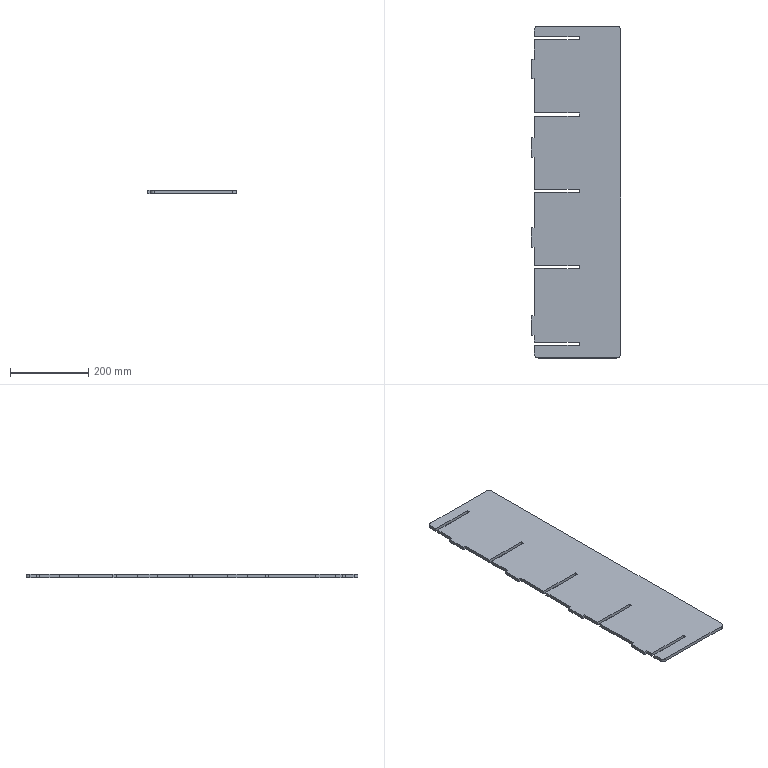Part | SolidWorks | features FlatPattern 1, SMBaseFlange 1, SheetMetal 1 | 1 solid | 46 faces | box 227.5 x 847.5 x 8 mm | volume 1466273 mm3 | plane 42 | cylinder 4 | commonest cylinder face diameters 20 x4
STEP:
#1=CARTESIAN_POINT('',(995.006,-468.438,0.));
#2=VERTEX_POINT('',#1);
#3=CARTESIAN_POINT('',(1005.006,-478.438,0.));
#4=VERTEX_POINT('',#3);
#5=CARTESIAN_POINT('',(1005.006,-468.438,0.));
#6=DIRECTION('',(0.,0.,1.));
#7=DIRECTION('',(-1.,0.,0.));
#8=AXIS2_PLACEMENT_3D('',#5,#6,#7);
#9=CIRCLE('',#8,10.);
#10=EDGE_CURVE('',#2,#4,#9,.T.);
#11=ORIENTED_EDGE('',*,*,#10,.F.);
#12=CARTESIAN_POINT('',(995.006,-468.438,-8.));
#13=VERTEX_POINT('',#12);
#14=CARTESIAN_POINT('',(995.006,-468.438,-8.));
#15=DIRECTION('',(0.,0.,1.));
#16=VECTOR('',#15,1000.);
#17=LINE('',#14,#16);
#18=EDGE_CURVE('',#13,#2,#17,.T.);
#19=ORIENTED_EDGE('',*,*,#18,.F.);
#20=CARTESIAN_POINT('',(1005.006,-478.438,-8.));
#21=VERTEX_POINT('',#20);
#22=CARTESIAN_POINT('',(1005.006,-468.438,-8.));
#23=DIRECTION('',(0.,0.,1.));
#24=DIRECTION('',(-1.,0.,0.));
#25=AXIS2_PLACEMENT_3D('',#22,#23,#24);
#26=CIRCLE('',#25,10.);
#27=EDGE_CURVE('',#13,#21,#26,.T.);
#28=ORIENTED_EDGE('',*,*,#27,.T.);
#29=CARTESIAN_POINT('',(1005.006,-478.438,-8.));
#30=DIRECTION('',(0.,0.,1.));
#31=VECTOR('',#30,1000.);
#32=LINE('',#29,#31);
#33=EDGE_CURVE('',#21,#4,#32,.T.);
#34=ORIENTED_EDGE('',*,*,#33,.T.);
#35=EDGE_LOOP('',(#11,#19,#28,#34));
#36=FACE_OUTER_BOUND('',#35,.T.);
#37=CARTESIAN_POINT('',(1005.006,-468.438,-8.));
#38=DIRECTION('',(0.,0.,1.));
#39=DIRECTION('',(1.,0.,0.));
#40=AXIS2_PLACEMENT_3D('',#37,#38,#39);
#41=CYLINDRICAL_SURFACE('',#40,10.);
#42=ADVANCED_FACE('',(#36),#41,.T.);
#43=CARTESIAN_POINT('',(995.006,-445.938,0.));
#44=VERTEX_POINT('',#43);
#45=CARTESIAN_POINT('',(995.006,-468.438,0.));
#46=DIRECTION('',(0.,-1.,0.));
#47=VECTOR('',#46,1000.);
#48=LINE('',#45,#47);
#49=EDGE_CURVE('',#44,#2,#48,.T.);
#50=ORIENTED_EDGE('',*,*,#49,.F.);
#51=CARTESIAN_POINT('',(995.006,-445.938,-8.));
#52=VERTEX_POINT('',#51);
#53=CARTESIAN_POINT('',(995.006,-445.938,-8.));
#54=DIRECTION('',(0.,0.,1.));
#55=VECTOR('',#54,1000.);
#56=LINE('',#53,#55);
#57=EDGE_CURVE('',#52,#44,#56,.T.);
#58=ORIENTED_EDGE('',*,*,#57,.F.);
#59=CARTESIAN_POINT('',(995.006,-468.438,-8.));
#60=DIRECTION('',(0.,-1.,0.));
#61=VECTOR('',#60,1000.);
#62=LINE('',#59,#61);
#63=EDGE_CURVE('',#52,#13,#62,.T.);
#64=ORIENTED_EDGE('',*,*,#63,.T.);
#65=ORIENTED_EDGE('',*,*,#18,.T.);
#66=EDGE_LOOP('',(#50,#58,#64,#65));
#67=FACE_OUTER_BOUND('',#66,.T.);
#68=CARTESIAN_POINT('',(995.006,-468.438,-8.));
#69=DIRECTION('',(-1.,0.,0.));
#70=DIRECTION('',(0.,-1.,0.));
#71=AXIS2_PLACEMENT_3D('',#68,#69,#70);
#72=PLANE('',#71);
#73=ADVANCED_FACE('',(#67),#72,.T.);
#74=CARTESIAN_POINT('',(1109.506,-445.938,0.));
#75=VERTEX_POINT('',#74);
#76=CARTESIAN_POINT('',(995.006,-445.938,0.));
#77=DIRECTION('',(-1.,0.,0.));
#78=VECTOR('',#77,1000.);
#79=LINE('',#76,#78);
#80=EDGE_CURVE('',#75,#44,#79,.T.);
#81=ORIENTED_EDGE('',*,*,#80,.F.);
#82=CARTESIAN_POINT('',(1109.506,-445.938,-8.));
#83=VERTEX_POINT('',#82);
#84=CARTESIAN_POINT('',(1109.506,-445.938,-8.));
#85=DIRECTION('',(0.,0.,1.));
#86=VECTOR('',#85,1000.);
#87=LINE('',#84,#86);
#88=EDGE_CURVE('',#83,#75,#87,.T.);
#89=ORIENTED_EDGE('',*,*,#88,.F.);
#90=CARTESIAN_POINT('',(995.006,-445.938,-8.));
#91=DIRECTION('',(-1.,0.,0.));
#92=VECTOR('',#91,1000.);
#93=LINE('',#90,#92);
#94=EDGE_CURVE('',#83,#52,#93,.T.);
#95=ORIENTED_EDGE('',*,*,#94,.T.);
#96=ORIENTED_EDGE('',*,*,#57,.T.);
#97=EDGE_LOOP('',(#81,#89,#95,#96));
#98=FACE_OUTER_BOUND('',#97,.T.);
#99=CARTESIAN_POINT('',(995.006,-445.938,-8.));
#100=DIRECTION('',(0.,1.,0.));
#101=DIRECTION('',(0.,0.,1.));
#102=AXIS2_PLACEMENT_3D('',#99,#100,#101);
#103=PLANE('',#102);
#104=ADVANCED_FACE('',(#98),#103,.T.);
#105=CARTESIAN_POINT('',(1109.506,-437.938,0.));
#106=VERTEX_POINT('',#105);
#107=CARTESIAN_POINT('',(1109.506,-445.938,0.));
#108=DIRECTION('',(0.,-1.,0.));
#109=VECTOR('',#108,1000.);
#110=LINE('',#107,#109);
#111=EDGE_CURVE('',#106,#75,#110,.T.);
#112=ORIENTED_EDGE('',*,*,#111,.F.);
#113=CARTESIAN_POINT('',(1109.506,-437.938,-8.));
#114=VERTEX_POINT('',#113);
#115=CARTESIAN_POINT('',(1109.506,-437.938,-8.));
#116=DIRECTION('',(0.,0.,1.));
#117=VECTOR('',#116,1000.);
#118=LINE('',#115,#117);
#119=EDGE_CURVE('',#114,#106,#118,.T.);
#120=ORIENTED_EDGE('',*,*,#119,.F.);
#121=CARTESIAN_POINT('',(1109.506,-445.938,-8.));
#122=DIRECTION('',(0.,-1.,0.));
#123=VECTOR('',#122,1000.);
#124=LINE('',#121,#123);
#125=EDGE_CURVE('',#114,#83,#124,.T.);
#126=ORIENTED_EDGE('',*,*,#125,.T.);
#127=ORIENTED_EDGE('',*,*,#88,.T.);
#128=EDGE_LOOP('',(#112,#120,#126,#127));
#129=FACE_OUTER_BOUND('',#128,.T.);
#130=CARTESIAN_POINT('',(1109.506,-445.938,-8.));
#131=DIRECTION('',(-1.,0.,0.));
#132=DIRECTION('',(0.,0.,1.));
#133=AXIS2_PLACEMENT_3D('',#130,#131,#132);
#134=PLANE('',#133);
#135=ADVANCED_FACE('',(#129),#134,.T.);
#136=CARTESIAN_POINT('',(995.006,-437.938,0.));
#137=VERTEX_POINT('',#136);
#138=CARTESIAN_POINT('',(1109.506,-437.938,0.));
#139=DIRECTION('',(1.,0.,0.));
#140=VECTOR('',#139,1000.);
#141=LINE('',#138,#140);
#142=EDGE_CURVE('',#137,#106,#141,.T.);
#143=ORIENTED_EDGE('',*,*,#142,.F.);
#144=CARTESIAN_POINT('',(995.006,-437.938,-8.));
#145=VERTEX_POINT('',#144);
#146=CARTESIAN_POINT('',(995.006,-437.938,-8.));
#147=DIRECTION('',(0.,0.,1.));
#148=VECTOR('',#147,1000.);
#149=LINE('',#146,#148);
#150=EDGE_CURVE('',#145,#137,#149,.T.);
#151=ORIENTED_EDGE('',*,*,#150,.F.);
#152=CARTESIAN_POINT('',(1109.506,-437.938,-8.));
#153=DIRECTION('',(1.,0.,0.));
#154=VECTOR('',#153,1000.);
#155=LINE('',#152,#154);
#156=EDGE_CURVE('',#145,#114,#155,.T.);
#157=ORIENTED_EDGE('',*,*,#156,.T.);
#158=ORIENTED_EDGE('',*,*,#119,.T.);
#159=EDGE_LOOP('',(#143,#151,#157,#158));
#160=FACE_OUTER_BOUND('',#159,.T.);
#161=CARTESIAN_POINT('',(1109.506,-437.938,-8.));
#162=DIRECTION('',(0.,-1.,0.));
#163=DIRECTION('',(0.,0.,-1.));
#164=AXIS2_PLACEMENT_3D('',#161,#162,#163);
#165=PLANE('',#164);
#166=ADVANCED_FACE('',(#160),#165,.T.);
#167=CARTESIAN_POINT('',(995.006,-420.938,0.));
#168=VERTEX_POINT('',#167);
#169=CARTESIAN_POINT('',(995.006,-437.938,0.));
#170=DIRECTION('',(0.,-1.,0.));
#171=VECTOR('',#170,1000.);
#172=LINE('',#169,#171);
#173=EDGE_CURVE('',#168,#137,#172,.T.);
#174=ORIENTED_EDGE('',*,*,#173,.F.);
#175=CARTESIAN_POINT('',(995.006,-420.938,-8.));
#176=VERTEX_POINT('',#175);
#177=CARTESIAN_POINT('',(995.006,-420.938,-8.));
#178=DIRECTION('',(0.,0.,1.));
#179=VECTOR('',#178,1000.);
#180=LINE('',#177,#179);
#181=EDGE_CURVE('',#176,#168,#180,.T.);
#182=ORIENTED_EDGE('',*,*,#181,.F.);
#183=CARTESIAN_POINT('',(995.006,-437.938,-8.));
#184=DIRECTION('',(0.,-1.,0.));
#185=VECTOR('',#184,1000.);
#186=LINE('',#183,#185);
#187=EDGE_CURVE('',#176,#145,#186,.T.);
#188=ORIENTED_EDGE('',*,*,#187,.T.);
#189=ORIENTED_EDGE('',*,*,#150,.T.);
#190=EDGE_LOOP('',(#174,#182,#188,#189));
#191=FACE_OUTER_BOUND('',#190,.T.);
#192=CARTESIAN_POINT('',(995.006,-437.938,-8.));
#193=DIRECTION('',(-1.,0.,0.));
#194=DIRECTION('',(0.,-1.,0.));
#195=AXIS2_PLACEMENT_3D('',#192,#193,#194);
#196=PLANE('',#195);
#197=ADVANCED_FACE('',(#191),#196,.T.);
#198=CARTESIAN_POINT('',(987.506,-420.938,0.));
#199=VERTEX_POINT('',#198);
#200=CARTESIAN_POINT('',(995.006,-420.938,0.));
#201=DIRECTION('',(1.,0.,0.));
#202=VECTOR('',#201,1000.);
#203=LINE('',#200,#202);
#204=EDGE_CURVE('',#199,#168,#203,.T.);
#205=ORIENTED_EDGE('',*,*,#204,.F.);
#206=CARTESIAN_POINT('',(987.506,-420.938,-8.));
#207=VERTEX_POINT('',#206);
#208=CARTESIAN_POINT('',(987.506,-420.938,-8.));
#209=DIRECTION('',(0.,0.,1.));
#210=VECTOR('',#209,1000.);
#211=LINE('',#208,#210);
#212=EDGE_CURVE('',#207,#199,#211,.T.);
#213=ORIENTED_EDGE('',*,*,#212,.F.);
#214=CARTESIAN_POINT('',(995.006,-420.938,-8.));
#215=DIRECTION('',(1.,0.,0.));
#216=VECTOR('',#215,1000.);
#217=LINE('',#214,#216);
#218=EDGE_CURVE('',#207,#176,#217,.T.);
#219=ORIENTED_EDGE('',*,*,#218,.T.);
#220=ORIENTED_EDGE('',*,*,#181,.T.);
#221=EDGE_LOOP('',(#205,#213,#219,#220));
#222=FACE_OUTER_BOUND('',#221,.T.);
#223=CARTESIAN_POINT('',(995.006,-420.938,-8.));
#224=DIRECTION('',(0.,-1.,0.));
#225=DIRECTION('',(0.,0.,-1.));
#226=AXIS2_PLACEMENT_3D('',#223,#224,#225);
#227=PLANE('',#226);
#228=ADVANCED_FACE('',(#222),#227,.T.);
#229=CARTESIAN_POINT('',(987.506,-370.938,0.));
#230=VERTEX_POINT('',#229);
#231=CARTESIAN_POINT('',(987.506,-420.938,0.));
#232=DIRECTION('',(0.,-1.,0.));
#233=VECTOR('',#232,1000.);
#234=LINE('',#231,#233);
#235=EDGE_CURVE('',#230,#199,#234,.T.);
#236=ORIENTED_EDGE('',*,*,#235,.F.);
#237=CARTESIAN_POINT('',(987.506,-370.938,-8.));
#238=VERTEX_POINT('',#237);
#239=CARTESIAN_POINT('',(987.506,-370.938,-8.));
#240=DIRECTION('',(0.,0.,1.));
#241=VECTOR('',#240,1000.);
#242=LINE('',#239,#241);
#243=EDGE_CURVE('',#238,#230,#242,.T.);
#244=ORIENTED_EDGE('',*,*,#243,.F.);
#245=CARTESIAN_POINT('',(987.506,-420.938,-8.));
#246=DIRECTION('',(0.,-1.,0.));
#247=VECTOR('',#246,1000.);
#248=LINE('',#245,#247);
#249=EDGE_CURVE('',#238,#207,#248,.T.);
#250=ORIENTED_EDGE('',*,*,#249,.T.);
#251=ORIENTED_EDGE('',*,*,#212,.T.);
#252=EDGE_LOOP('',(#236,#244,#250,#251));
#253=FACE_OUTER_BOUND('',#252,.T.);
#254=CARTESIAN_POINT('',(987.506,-420.938,-8.));
#255=DIRECTION('',(-1.,0.,0.));
#256=DIRECTION('',(0.,0.,1.));
#257=AXIS2_PLACEMENT_3D('',#254,#255,#256);
#258=PLANE('',#257);
#259=ADVANCED_FACE('',(#253),#258,.T.);
#260=CARTESIAN_POINT('',(995.006,-370.938,0.));
#261=VERTEX_POINT('',#260);
#262=CARTESIAN_POINT('',(987.506,-370.938,0.));
#263=DIRECTION('',(-1.,0.,0.));
#264=VECTOR('',#263,1000.);
#265=LINE('',#262,#264);
#266=EDGE_CURVE('',#261,#230,#265,.T.);
#267=ORIENTED_EDGE('',*,*,#266,.F.);
#268=CARTESIAN_POINT('',(995.006,-370.938,-8.));
#269=VERTEX_POINT('',#268);
#270=CARTESIAN_POINT('',(995.006,-370.938,-8.));
#271=DIRECTION('',(0.,0.,1.));
#272=VECTOR('',#271,1000.);
#273=LINE('',#270,#272);
#274=EDGE_CURVE('',#269,#261,#273,.T.);
#275=ORIENTED_EDGE('',*,*,#274,.F.);
#276=CARTESIAN_POINT('',(987.506,-370.938,-8.));
#277=DIRECTION('',(-1.,0.,0.));
#278=VECTOR('',#277,1000.);
#279=LINE('',#276,#278);
#280=EDGE_CURVE('',#269,#238,#279,.T.);
#281=ORIENTED_EDGE('',*,*,#280,.T.);
#282=ORIENTED_EDGE('',*,*,#243,.T.);
#283=EDGE_LOOP('',(#267,#275,#281,#282));
#284=FACE_OUTER_BOUND('',#283,.T.);
#285=CARTESIAN_POINT('',(987.506,-370.938,-8.));
#286=DIRECTION('',(0.,1.,0.));
#287=DIRECTION('',(0.,0.,1.));
#288=AXIS2_PLACEMENT_3D('',#285,#286,#287);
#289=PLANE('',#288);
#290=ADVANCED_FACE('',(#284),#289,.T.);
#291=CARTESIAN_POINT('',(995.006,-250.938,0.));
#292=VERTEX_POINT('',#291);
#293=CARTESIAN_POINT('',(995.006,-370.938,0.));
#294=DIRECTION('',(0.,-1.,0.));
#295=VECTOR('',#294,1000.);
#296=LINE('',#293,#295);
#297=EDGE_CURVE('',#292,#261,#296,.T.);
#298=ORIENTED_EDGE('',*,*,#297,.F.);
#299=CARTESIAN_POINT('',(995.006,-250.938,-8.));
#300=VERTEX_POINT('',#299);
#301=CARTESIAN_POINT('',(995.006,-250.938,-8.));
#302=DIRECTION('',(0.,0.,1.));
#303=VECTOR('',#302,1000.);
#304=LINE('',#301,#303);
#305=EDGE_CURVE('',#300,#292,#304,.T.);
#306=ORIENTED_EDGE('',*,*,#305,.F.);
#307=CARTESIAN_POINT('',(995.006,-370.938,-8.));
#308=DIRECTION('',(0.,-1.,0.));
#309=VECTOR('',#308,1000.);
#310=LINE('',#307,#309);
#311=EDGE_CURVE('',#300,#269,#310,.T.);
#312=ORIENTED_EDGE('',*,*,#311,.T.);
#313=ORIENTED_EDGE('',*,*,#274,.T.);
#314=EDGE_LOOP('',(#298,#306,#312,#313));
#315=FACE_OUTER_BOUND('',#314,.T.);
#316=CARTESIAN_POINT('',(995.006,-370.938,-8.));
#317=DIRECTION('',(-1.,0.,0.));
#318=DIRECTION('',(0.,-1.,0.));
#319=AXIS2_PLACEMENT_3D('',#316,#317,#318);
#320=PLANE('',#319);
#321=ADVANCED_FACE('',(#315),#320,.T.);
#322=CARTESIAN_POINT('',(1109.506,-250.938,0.));
#323=VERTEX_POINT('',#322);
#324=CARTESIAN_POINT('',(995.006,-250.938,0.));
#325=DIRECTION('',(-1.,0.,0.));
#326=VECTOR('',#325,1000.);
#327=LINE('',#324,#326);
#328=EDGE_CURVE('',#323,#292,#327,.T.);
#329=ORIENTED_EDGE('',*,*,#328,.F.);
#330=CARTESIAN_POINT('',(1109.506,-250.938,-8.));
#331=VERTEX_POINT('',#330);
#332=CARTESIAN_POINT('',(1109.506,-250.938,-8.));
#333=DIRECTION('',(0.,0.,1.));
#334=VECTOR('',#333,1000.);
#335=LINE('',#332,#334);
#336=EDGE_CURVE('',#331,#323,#335,.T.);
#337=ORIENTED_EDGE('',*,*,#336,.F.);
#338=CARTESIAN_POINT('',(995.006,-250.938,-8.));
#339=DIRECTION('',(-1.,0.,0.));
#340=VECTOR('',#339,1000.);
#341=LINE('',#338,#340);
#342=EDGE_CURVE('',#331,#300,#341,.T.);
#343=ORIENTED_EDGE('',*,*,#342,.T.);
#344=ORIENTED_EDGE('',*,*,#305,.T.);
#345=EDGE_LOOP('',(#329,#337,#343,#344));
#346=FACE_OUTER_BOUND('',#345,.T.);
#347=CARTESIAN_POINT('',(995.006,-250.938,-8.));
#348=DIRECTION('',(0.,1.,0.));
#349=DIRECTION('',(0.,0.,1.));
#350=AXIS2_PLACEMENT_3D('',#347,#348,#349);
#351=PLANE('',#350);
#352=ADVANCED_FACE('',(#346),#351,.T.);
#353=CARTESIAN_POINT('',(1109.506,-242.938,0.));
#354=VERTEX_POINT('',#353);
#355=CARTESIAN_POINT('',(1109.506,-250.938,0.));
#356=DIRECTION('',(0.,-1.,0.));
#357=VECTOR('',#356,1000.);
#358=LINE('',#355,#357);
#359=EDGE_CURVE('',#354,#323,#358,.T.);
#360=ORIENTED_EDGE('',*,*,#359,.F.);
#361=CARTESIAN_POINT('',(1109.506,-242.938,-8.));
#362=VERTEX_POINT('',#361);
#363=CARTESIAN_POINT('',(1109.506,-242.938,-8.));
#364=DIRECTION('',(0.,0.,1.));
#365=VECTOR('',#364,1000.);
#366=LINE('',#363,#365);
#367=EDGE_CURVE('',#362,#354,#366,.T.);
#368=ORIENTED_EDGE('',*,*,#367,.F.);
#369=CARTESIAN_POINT('',(1109.506,-250.938,-8.));
#370=DIRECTION('',(0.,-1.,0.));
#371=VECTOR('',#370,1000.);
#372=LINE('',#369,#371);
#373=EDGE_CURVE('',#362,#331,#372,.T.);
#374=ORIENTED_EDGE('',*,*,#373,.T.);
#375=ORIENTED_EDGE('',*,*,#336,.T.);
#376=EDGE_LOOP('',(#360,#368,#374,#375));
#377=FACE_OUTER_BOUND('',#376,.T.);
#378=CARTESIAN_POINT('',(1109.506,-250.938,-8.));
#379=DIRECTION('',(-1.,0.,0.));
#380=DIRECTION('',(0.,0.,1.));
#381=AXIS2_PLACEMENT_3D('',#378,#379,#380);
#382=PLANE('',#381);
#383=ADVANCED_FACE('',(#377),#382,.T.);
#384=CARTESIAN_POINT('',(995.006,-242.938,0.));
#385=VERTEX_POINT('',#384);
#386=CARTESIAN_POINT('',(1109.506,-242.938,0.));
#387=DIRECTION('',(1.,0.,0.));
#388=VECTOR('',#387,1000.);
#389=LINE('',#386,#388);
#390=EDGE_CURVE('',#385,#354,#389,.T.);
#391=ORIENTED_EDGE('',*,*,#390,.F.);
#392=CARTESIAN_POINT('',(995.006,-242.938,-8.));
#393=VERTEX_POINT('',#392);
#394=CARTESIAN_POINT('',(995.006,-242.938,-8.));
#395=DIRECTION('',(0.,0.,1.));
#396=VECTOR('',#395,1000.);
#397=LINE('',#394,#396);
#398=EDGE_CURVE('',#393,#385,#397,.T.);
#399=ORIENTED_EDGE('',*,*,#398,.F.);
#400=CARTESIAN_POINT('',(1109.506,-242.938,-8.));
#401=DIRECTION('',(1.,0.,0.));
#402=VECTOR('',#401,1000.);
#403=LINE('',#400,#402);
#404=EDGE_CURVE('',#393,#362,#403,.T.);
#405=ORIENTED_EDGE('',*,*,#404,.T.);
#406=ORIENTED_EDGE('',*,*,#367,.T.);
#407=EDGE_LOOP('',(#391,#399,#405,#406));
#408=FACE_OUTER_BOUND('',#407,.T.);
#409=CARTESIAN_POINT('',(1109.506,-242.938,-8.));
#410=DIRECTION('',(0.,-1.,0.));
#411=DIRECTION('',(0.,0.,-1.));
#412=AXIS2_PLACEMENT_3D('',#409,#410,#411);
#413=PLANE('',#412);
#414=ADVANCED_FACE('',(#408),#413,.T.);
#415=CARTESIAN_POINT('',(995.006,-195.938,0.));
#416=VERTEX_POINT('',#415);
#417=CARTESIAN_POINT('',(995.006,-242.938,0.));
#418=DIRECTION('',(0.,-1.,0.));
#419=VECTOR('',#418,1000.);
#420=LINE('',#417,#419);
#421=EDGE_CURVE('',#416,#385,#420,.T.);
#422=ORIENTED_EDGE('',*,*,#421,.F.);
#423=CARTESIAN_POINT('',(995.006,-195.938,-8.));
#424=VERTEX_POINT('',#423);
#425=CARTESIAN_POINT('',(995.006,-195.938,-8.));
#426=DIRECTION('',(0.,0.,1.));
#427=VECTOR('',#426,1000.);
#428=LINE('',#425,#427);
#429=EDGE_CURVE('',#424,#416,#428,.T.);
#430=ORIENTED_EDGE('',*,*,#429,.F.);
#431=CARTESIAN_POINT('',(995.006,-242.938,-8.));
#432=DIRECTION('',(0.,-1.,0.));
#433=VECTOR('',#432,1000.);
#434=LINE('',#431,#433);
#435=EDGE_CURVE('',#424,#393,#434,.T.);
#436=ORIENTED_EDGE('',*,*,#435,.T.);
#437=ORIENTED_EDGE('',*,*,#398,.T.);
#438=EDGE_LOOP('',(#422,#430,#436,#437));
#439=FACE_OUTER_BOUND('',#438,.T.);
#440=CARTESIAN_POINT('',(995.006,-242.938,-8.));
#441=DIRECTION('',(-1.,0.,0.));
#442=DIRECTION('',(0.,-1.,0.));
#443=AXIS2_PLACEMENT_3D('',#440,#441,#442);
#444=PLANE('',#443);
#445=ADVANCED_FACE('',(#439),#444,.T.);
#446=CARTESIAN_POINT('',(987.506,-195.938,0.));
#447=VERTEX_POINT('',#446);
#448=CARTESIAN_POINT('',(995.006,-195.938,0.));
#449=DIRECTION('',(1.,0.,0.));
#450=VECTOR('',#449,1000.);
#451=LINE('',#448,#450);
#452=EDGE_CURVE('',#447,#416,#451,.T.);
#453=ORIENTED_EDGE('',*,*,#452,.F.);
#454=CARTESIAN_POINT('',(987.506,-195.938,-8.));
#455=VERTEX_POINT('',#454);
#456=CARTESIAN_POINT('',(987.506,-195.938,-8.));
#457=DIRECTION('',(0.,0.,1.));
#458=VECTOR('',#457,1000.);
#459=LINE('',#456,#458);
#460=EDGE_CURVE('',#455,#447,#459,.T.);
#461=ORIENTED_EDGE('',*,*,#460,.F.);
#462=CARTESIAN_POINT('',(995.006,-195.938,-8.));
#463=DIRECTION('',(1.,0.,0.));
#464=VECTOR('',#463,1000.);
#465=LINE('',#462,#464);
#466=EDGE_CURVE('',#455,#424,#465,.T.);
#467=ORIENTED_EDGE('',*,*,#466,.T.);
#468=ORIENTED_EDGE('',*,*,#429,.T.);
#469=EDGE_LOOP('',(#453,#461,#467,#468));
#470=FACE_OUTER_BOUND('',#469,.T.);
#471=CARTESIAN_POINT('',(995.006,-195.938,-8.));
#472=DIRECTION('',(0.,-1.,0.));
#473=DIRECTION('',(1.,0.,0.));
#474=AXIS2_PLACEMENT_3D('',#471,#472,#473);
#475=PLANE('',#474);
#476=ADVANCED_FACE('',(#470),#475,.T.);
#477=CARTESIAN_POINT('',(987.506,-145.938,0.));
#478=VERTEX_POINT('',#477);
#479=CARTESIAN_POINT('',(987.506,-195.938,0.));
#480=DIRECTION('',(0.,-1.,0.));
#481=VECTOR('',#480,1000.);
#482=LINE('',#479,#481);
#483=EDGE_CURVE('',#478,#447,#482,.T.);
#484=ORIENTED_EDGE('',*,*,#483,.F.);
#485=CARTESIAN_POINT('',(987.506,-145.938,-8.));
#486=VERTEX_POINT('',#485);
#487=CARTESIAN_POINT('',(987.506,-145.938,-8.));
#488=DIRECTION('',(0.,0.,1.));
#489=VECTOR('',#488,1000.);
#490=LINE('',#487,#489);
#491=EDGE_CURVE('',#486,#478,#490,.T.);
#492=ORIENTED_EDGE('',*,*,#491,.F.);
#493=CARTESIAN_POINT('',(987.506,-195.938,-8.));
#494=DIRECTION('',(0.,-1.,0.));
#495=VECTOR('',#494,1000.);
#496=LINE('',#493,#495);
#497=EDGE_CURVE('',#486,#455,#496,.T.);
#498=ORIENTED_EDGE('',*,*,#497,.T.);
#499=ORIENTED_EDGE('',*,*,#460,.T.);
#500=EDGE_LOOP('',(#484,#492,#498,#499));
#501=FACE_OUTER_BOUND('',#500,.T.);
#502=CARTESIAN_POINT('',(987.506,-195.938,-8.));
#503=DIRECTION('',(-1.,0.,0.));
#504=DIRECTION('',(0.,0.,1.));
#505=AXIS2_PLACEMENT_3D('',#502,#503,#504);
#506=PLANE('',#505);
#507=ADVANCED_FACE('',(#501),#506,.T.);
#508=CARTESIAN_POINT('',(995.006,-145.938,0.));
#509=VERTEX_POINT('',#508);
#510=CARTESIAN_POINT('',(987.506,-145.938,0.));
#511=DIRECTION('',(-1.,0.,0.));
#512=VECTOR('',#511,1000.);
#513=LINE('',#510,#512);
#514=EDGE_CURVE('',#509,#478,#513,.T.);
#515=ORIENTED_EDGE('',*,*,#514,.F.);
#516=CARTESIAN_POINT('',(995.006,-145.938,-8.));
#517=VERTEX_POINT('',#516);
#518=CARTESIAN_POINT('',(995.006,-145.938,-8.));
#519=DIRECTION('',(0.,0.,1.));
#520=VECTOR('',#519,1000.);
#521=LINE('',#518,#520);
#522=EDGE_CURVE('',#517,#509,#521,.T.);
#523=ORIENTED_EDGE('',*,*,#522,.F.);
#524=CARTESIAN_POINT('',(987.506,-145.938,-8.));
#525=DIRECTION('',(-1.,0.,0.));
#526=VECTOR('',#525,1000.);
#527=LINE('',#524,#526);
#528=EDGE_CURVE('',#517,#486,#527,.T.);
#529=ORIENTED_EDGE('',*,*,#528,.T.);
#530=ORIENTED_EDGE('',*,*,#491,.T.);
#531=EDGE_LOOP('',(#515,#523,#529,#530));
#532=FACE_OUTER_BOUND('',#531,.T.);
#533=CARTESIAN_POINT('',(987.506,-145.938,-8.));
#534=DIRECTION('',(0.,1.,0.));
#535=DIRECTION('',(0.,0.,1.));
#536=AXIS2_PLACEMENT_3D('',#533,#534,#535);
#537=PLANE('',#536);
#538=ADVANCED_FACE('',(#532),#537,.T.);
#539=CARTESIAN_POINT('',(995.006,-55.938,0.));
#540=VERTEX_POINT('',#539);
#541=CARTESIAN_POINT('',(995.006,-145.938,0.));
#542=DIRECTION('',(0.,-1.,0.));
#543=VECTOR('',#542,1000.);
#544=LINE('',#541,#543);
#545=EDGE_CURVE('',#540,#509,#544,.T.);
#546=ORIENTED_EDGE('',*,*,#545,.F.);
#547=CARTESIAN_POINT('',(995.006,-55.938,-8.));
#548=VERTEX_POINT('',#547);
#549=CARTESIAN_POINT('',(995.006,-55.938,-8.));
#550=DIRECTION('',(0.,0.,1.));
#551=VECTOR('',#550,1000.);
#552=LINE('',#549,#551);
#553=EDGE_CURVE('',#548,#540,#552,.T.);
#554=ORIENTED_EDGE('',*,*,#553,.F.);
#555=CARTESIAN_POINT('',(995.006,-145.938,-8.));
#556=DIRECTION('',(0.,-1.,0.));
#557=VECTOR('',#556,1000.);
#558=LINE('',#555,#557);
#559=EDGE_CURVE('',#548,#517,#558,.T.);
#560=ORIENTED_EDGE('',*,*,#559,.T.);
#561=ORIENTED_EDGE('',*,*,#522,.T.);
#562=EDGE_LOOP('',(#546,#554,#560,#561));
#563=FACE_OUTER_BOUND('',#562,.T.);
#564=CARTESIAN_POINT('',(995.006,-145.938,-8.));
#565=DIRECTION('',(-1.,0.,0.));
#566=DIRECTION('',(0.,-1.,0.));
#567=AXIS2_PLACEMENT_3D('',#564,#565,#566);
#568=PLANE('',#567);
#569=ADVANCED_FACE('',(#563),#568,.T.);
#570=CARTESIAN_POINT('',(1109.506,-55.938,0.));
#571=VERTEX_POINT('',#570);
#572=CARTESIAN_POINT('',(995.006,-55.938,0.));
#573=DIRECTION('',(-1.,0.,0.));
#574=VECTOR('',#573,1000.);
#575=LINE('',#572,#574);
#576=EDGE_CURVE('',#571,#540,#575,.T.);
#577=ORIENTED_EDGE('',*,*,#576,.F.);
#578=CARTESIAN_POINT('',(1109.506,-55.938,-8.));
#579=VERTEX_POINT('',#578);
#580=CARTESIAN_POINT('',(1109.506,-55.938,-8.));
#581=DIRECTION('',(0.,0.,1.));
#582=VECTOR('',#581,1000.);
#583=LINE('',#580,#582);
#584=EDGE_CURVE('',#579,#571,#583,.T.);
#585=ORIENTED_EDGE('',*,*,#584,.F.);
#586=CARTESIAN_POINT('',(995.006,-55.938,-8.));
#587=DIRECTION('',(-1.,0.,0.));
#588=VECTOR('',#587,1000.);
#589=LINE('',#586,#588);
#590=EDGE_CURVE('',#579,#548,#589,.T.);
#591=ORIENTED_EDGE('',*,*,#590,.T.);
#592=ORIENTED_EDGE('',*,*,#553,.T.);
#593=EDGE_LOOP('',(#577,#585,#591,#592));
#594=FACE_OUTER_BOUND('',#593,.T.);
#595=CARTESIAN_POINT('',(995.006,-55.938,-8.));
#596=DIRECTION('',(0.,1.,0.));
#597=DIRECTION('',(0.,0.,1.));
#598=AXIS2_PLACEMENT_3D('',#595,#596,#597);
#599=PLANE('',#598);
#600=ADVANCED_FACE('',(#594),#599,.T.);
#601=CARTESIAN_POINT('',(1109.506,-47.938,0.));
#602=VERTEX_POINT('',#601);
#603=CARTESIAN_POINT('',(1109.506,-55.938,0.));
#604=DIRECTION('',(0.,-1.,0.));
#605=VECTOR('',#604,1000.);
#606=LINE('',#603,#605);
#607=EDGE_CURVE('',#602,#571,#606,.T.);
#608=ORIENTED_EDGE('',*,*,#607,.F.);
#609=CARTESIAN_POINT('',(1109.506,-47.938,-8.));
#610=VERTEX_POINT('',#609);
#611=CARTESIAN_POINT('',(1109.506,-47.938,-8.));
#612=DIRECTION('',(0.,0.,1.));
#613=VECTOR('',#612,1000.);
#614=LINE('',#611,#613);
#615=EDGE_CURVE('',#610,#602,#614,.T.);
#616=ORIENTED_EDGE('',*,*,#615,.F.);
#617=CARTESIAN_POINT('',(1109.506,-55.938,-8.));
#618=DIRECTION('',(0.,-1.,0.));
#619=VECTOR('',#618,1000.);
#620=LINE('',#617,#619);
#621=EDGE_CURVE('',#610,#579,#620,.T.);
#622=ORIENTED_EDGE('',*,*,#621,.T.);
#623=ORIENTED_EDGE('',*,*,#584,.T.);
#624=EDGE_LOOP('',(#608,#616,#622,#623));
#625=FACE_OUTER_BOUND('',#624,.T.);
#626=CARTESIAN_POINT('',(1109.506,-55.938,-8.));
#627=DIRECTION('',(-1.,0.,0.));
#628=DIRECTION('',(0.,0.,1.));
#629=AXIS2_PLACEMENT_3D('',#626,#627,#628);
#630=PLANE('',#629);
#631=ADVANCED_FACE('',(#625),#630,.T.);
#632=CARTESIAN_POINT('',(995.006,-47.938,0.));
#633=VERTEX_POINT('',#632);
#634=CARTESIAN_POINT('',(1109.506,-47.938,0.));
#635=DIRECTION('',(1.,0.,0.));
#636=VECTOR('',#635,1000.);
#637=LINE('',#634,#636);
#638=EDGE_CURVE('',#633,#602,#637,.T.);
#639=ORIENTED_EDGE('',*,*,#638,.F.);
#640=CARTESIAN_POINT('',(995.006,-47.938,-8.));
#641=VERTEX_POINT('',#640);
#642=CARTESIAN_POINT('',(995.006,-47.938,-8.));
#643=DIRECTION('',(0.,0.,1.));
#644=VECTOR('',#643,1000.);
#645=LINE('',#642,#644);
#646=EDGE_CURVE('',#641,#633,#645,.T.);
#647=ORIENTED_EDGE('',*,*,#646,.F.);
#648=CARTESIAN_POINT('',(1109.506,-47.938,-8.));
#649=DIRECTION('',(1.,0.,0.));
#650=VECTOR('',#649,1000.);
#651=LINE('',#648,#650);
#652=EDGE_CURVE('',#641,#610,#651,.T.);
#653=ORIENTED_EDGE('',*,*,#652,.T.);
#654=ORIENTED_EDGE('',*,*,#615,.T.);
#655=EDGE_LOOP('',(#639,#647,#653,#654));
#656=FACE_OUTER_BOUND('',#655,.T.);
#657=CARTESIAN_POINT('',(1109.506,-47.938,-8.));
#658=DIRECTION('',(0.,-1.,0.));
#659=DIRECTION('',(1.,0.,0.));
#660=AXIS2_PLACEMENT_3D('',#657,#658,#659);
#661=PLANE('',#660);
#662=ADVANCED_FACE('',(#656),#661,.T.);
#663=CARTESIAN_POINT('',(995.006,34.062,0.));
#664=VERTEX_POINT('',#663);
#665=CARTESIAN_POINT('',(995.006,-47.938,0.));
#666=DIRECTION('',(0.,-1.,0.));
#667=VECTOR('',#666,1000.);
#668=LINE('',#665,#667);
#669=EDGE_CURVE('',#664,#633,#668,.T.);
#670=ORIENTED_EDGE('',*,*,#669,.F.);
#671=CARTESIAN_POINT('',(995.006,34.062,-8.));
#672=VERTEX_POINT('',#671);
#673=CARTESIAN_POINT('',(995.006,34.062,-8.));
#674=DIRECTION('',(0.,0.,1.));
#675=VECTOR('',#674,1000.);
#676=LINE('',#673,#675);
#677=EDGE_CURVE('',#672,#664,#676,.T.);
#678=ORIENTED_EDGE('',*,*,#677,.F.);
#679=CARTESIAN_POINT('',(995.006,-47.938,-8.));
#680=DIRECTION('',(0.,-1.,0.));
#681=VECTOR('',#680,1000.);
#682=LINE('',#679,#681);
#683=EDGE_CURVE('',#672,#641,#682,.T.);
#684=ORIENTED_EDGE('',*,*,#683,.T.);
#685=ORIENTED_EDGE('',*,*,#646,.T.);
#686=EDGE_LOOP('',(#670,#678,#684,#685));
#687=FACE_OUTER_BOUND('',#686,.T.);
#688=CARTESIAN_POINT('',(995.006,-47.938,-8.));
#689=DIRECTION('',(-1.,0.,0.));
#690=DIRECTION('',(0.,-1.,0.));
#691=AXIS2_PLACEMENT_3D('',#688,#689,#690);
#692=PLANE('',#691);
#693=ADVANCED_FACE('',(#687),#692,.T.);
#694=CARTESIAN_POINT('',(987.506,34.062,0.));
#695=VERTEX_POINT('',#694);
#696=CARTESIAN_POINT('',(995.006,34.062,0.));
#697=DIRECTION('',(1.,0.,0.));
#698=VECTOR('',#697,1000.);
#699=LINE('',#696,#698);
#700=EDGE_CURVE('',#695,#664,#699,.T.);
#701=ORIENTED_EDGE('',*,*,#700,.F.);
#702=CARTESIAN_POINT('',(987.506,34.062,-8.));
#703=VERTEX_POINT('',#702);
#704=CARTESIAN_POINT('',(987.506,34.062,-8.));
#705=DIRECTION('',(0.,0.,1.));
#706=VECTOR('',#705,1000.);
#707=LINE('',#704,#706);
#708=EDGE_CURVE('',#703,#695,#707,.T.);
#709=ORIENTED_EDGE('',*,*,#708,.F.);
#710=CARTESIAN_POINT('',(995.006,34.062,-8.));
#711=DIRECTION('',(1.,0.,0.));
#712=VECTOR('',#711,1000.);
#713=LINE('',#710,#712);
#714=EDGE_CURVE('',#703,#672,#713,.T.);
#715=ORIENTED_EDGE('',*,*,#714,.T.);
#716=ORIENTED_EDGE('',*,*,#677,.T.);
#717=EDGE_LOOP('',(#701,#709,#715,#716));
#718=FACE_OUTER_BOUND('',#717,.T.);
#719=CARTESIAN_POINT('',(995.006,34.062,-8.));
#720=DIRECTION('',(0.,-1.,0.));
#721=DIRECTION('',(1.,0.,0.));
#722=AXIS2_PLACEMENT_3D('',#719,#720,#721);
#723=PLANE('',#722);
#724=ADVANCED_FACE('',(#718),#723,.T.);
#725=CARTESIAN_POINT('',(987.506,84.062,0.));
#726=VERTEX_POINT('',#725);
#727=CARTESIAN_POINT('',(987.506,34.062,0.));
#728=DIRECTION('',(0.,-1.,0.));
#729=VECTOR('',#728,1000.);
#730=LINE('',#727,#729);
#731=EDGE_CURVE('',#726,#695,#730,.T.);
#732=ORIENTED_EDGE('',*,*,#731,.F.);
#733=CARTESIAN_POINT('',(987.506,84.062,-8.));
#734=VERTEX_POINT('',#733);
#735=CARTESIAN_POINT('',(987.506,84.062,-8.));
#736=DIRECTION('',(0.,0.,1.));
#737=VECTOR('',#736,1000.);
#738=LINE('',#735,#737);
#739=EDGE_CURVE('',#734,#726,#738,.T.);
#740=ORIENTED_EDGE('',*,*,#739,.F.);
#741=CARTESIAN_POINT('',(987.506,34.062,-8.));
#742=DIRECTION('',(0.,-1.,0.));
#743=VECTOR('',#742,1000.);
#744=LINE('',#741,#743);
#745=EDGE_CURVE('',#734,#703,#744,.T.);
#746=ORIENTED_EDGE('',*,*,#745,.T.);
#747=ORIENTED_EDGE('',*,*,#708,.T.);
#748=EDGE_LOOP('',(#732,#740,#746,#747));
#749=FACE_OUTER_BOUND('',#748,.T.);
#750=CARTESIAN_POINT('',(987.506,34.062,-8.));
#751=DIRECTION('',(-1.,0.,0.));
#752=DIRECTION('',(0.,0.,1.));
#753=AXIS2_PLACEMENT_3D('',#750,#751,#752);
#754=PLANE('',#753);
#755=ADVANCED_FACE('',(#749),#754,.T.);
#756=CARTESIAN_POINT('',(995.006,84.062,0.));
#757=VERTEX_POINT('',#756);
#758=CARTESIAN_POINT('',(987.506,84.062,0.));
#759=DIRECTION('',(-1.,0.,0.));
#760=VECTOR('',#759,1000.);
#761=LINE('',#758,#760);
#762=EDGE_CURVE('',#757,#726,#761,.T.);
#763=ORIENTED_EDGE('',*,*,#762,.F.);
#764=CARTESIAN_POINT('',(995.006,84.062,-8.));
#765=VERTEX_POINT('',#764);
#766=CARTESIAN_POINT('',(995.006,84.062,-8.));
#767=DIRECTION('',(0.,0.,1.));
#768=VECTOR('',#767,1000.);
#769=LINE('',#766,#768);
#770=EDGE_CURVE('',#765,#757,#769,.T.);
#771=ORIENTED_EDGE('',*,*,#770,.F.);
#772=CARTESIAN_POINT('',(987.506,84.062,-8.));
#773=DIRECTION('',(-1.,0.,0.));
#774=VECTOR('',#773,1000.);
#775=LINE('',#772,#774);
#776=EDGE_CURVE('',#765,#734,#775,.T.);
#777=ORIENTED_EDGE('',*,*,#776,.T.);
#778=ORIENTED_EDGE('',*,*,#739,.T.);
#779=EDGE_LOOP('',(#763,#771,#777,#778));
#780=FACE_OUTER_BOUND('',#779,.T.);
#781=CARTESIAN_POINT('',(987.506,84.062,-8.));
#782=DIRECTION('',(0.,1.,0.));
#783=DIRECTION('',(-1.,0.,0.));
#784=AXIS2_PLACEMENT_3D('',#781,#782,#783);
#785=PLANE('',#784);
#786=ADVANCED_FACE('',(#780),#785,.T.);
#787=CARTESIAN_POINT('',(995.006,139.062,0.));
#788=VERTEX_POINT('',#787);
#789=CARTESIAN_POINT('',(995.006,84.062,0.));
#790=DIRECTION('',(0.,-1.,0.));
#791=VECTOR('',#790,1000.);
#792=LINE('',#789,#791);
#793=EDGE_CURVE('',#788,#757,#792,.T.);
#794=ORIENTED_EDGE('',*,*,#793,.F.);
#795=CARTESIAN_POINT('',(995.006,139.062,-8.));
#796=VERTEX_POINT('',#795);
#797=CARTESIAN_POINT('',(995.006,139.062,-8.));
#798=DIRECTION('',(0.,0.,1.));
#799=VECTOR('',#798,1000.);
#800=LINE('',#797,#799);
#801=EDGE_CURVE('',#796,#788,#800,.T.);
#802=ORIENTED_EDGE('',*,*,#801,.F.);
#803=CARTESIAN_POINT('',(995.006,84.062,-8.));
#804=DIRECTION('',(0.,-1.,0.));
#805=VECTOR('',#804,1000.);
#806=LINE('',#803,#805);
#807=EDGE_CURVE('',#796,#765,#806,.T.);
#808=ORIENTED_EDGE('',*,*,#807,.T.);
#809=ORIENTED_EDGE('',*,*,#770,.T.);
#810=EDGE_LOOP('',(#794,#802,#808,#809));
#811=FACE_OUTER_BOUND('',#810,.T.);
#812=CARTESIAN_POINT('',(995.006,84.062,-8.));
#813=DIRECTION('',(-1.,0.,0.));
#814=DIRECTION('',(0.,-1.,0.));
#815=AXIS2_PLACEMENT_3D('',#812,#813,#814);
#816=PLANE('',#815);
#817=ADVANCED_FACE('',(#811),#816,.T.);
#818=CARTESIAN_POINT('',(1109.506,139.062,0.));
#819=VERTEX_POINT('',#818);
#820=CARTESIAN_POINT('',(995.006,139.062,0.));
#821=DIRECTION('',(-1.,0.,0.));
#822=VECTOR('',#821,1000.);
#823=LINE('',#820,#822);
#824=EDGE_CURVE('',#819,#788,#823,.T.);
#825=ORIENTED_EDGE('',*,*,#824,.F.);
#826=CARTESIAN_POINT('',(1109.506,139.062,-8.));
#827=VERTEX_POINT('',#826);
#828=CARTESIAN_POINT('',(1109.506,139.062,-8.));
#829=DIRECTION('',(0.,0.,1.));
#830=VECTOR('',#829,1000.);
#831=LINE('',#828,#830);
#832=EDGE_CURVE('',#827,#819,#831,.T.);
#833=ORIENTED_EDGE('',*,*,#832,.F.);
#834=CARTESIAN_POINT('',(995.006,139.062,-8.));
#835=DIRECTION('',(-1.,0.,0.));
#836=VECTOR('',#835,1000.);
#837=LINE('',#834,#836);
#838=EDGE_CURVE('',#827,#796,#837,.T.);
#839=ORIENTED_EDGE('',*,*,#838,.T.);
#840=ORIENTED_EDGE('',*,*,#801,.T.);
#841=EDGE_LOOP('',(#825,#833,#839,#840));
#842=FACE_OUTER_BOUND('',#841,.T.);
#843=CARTESIAN_POINT('',(995.006,139.062,-8.));
#844=DIRECTION('',(0.,1.,0.));
#845=DIRECTION('',(0.,0.,1.));
#846=AXIS2_PLACEMENT_3D('',#843,#844,#845);
#847=PLANE('',#846);
#848=ADVANCED_FACE('',(#842),#847,.T.);
#849=CARTESIAN_POINT('',(1109.506,147.062,0.));
#850=VERTEX_POINT('',#849);
#851=CARTESIAN_POINT('',(1109.506,139.062,0.));
#852=DIRECTION('',(0.,-1.,0.));
#853=VECTOR('',#852,1000.);
#854=LINE('',#851,#853);
#855=EDGE_CURVE('',#850,#819,#854,.T.);
#856=ORIENTED_EDGE('',*,*,#855,.F.);
#857=CARTESIAN_POINT('',(1109.506,147.062,-8.));
#858=VERTEX_POINT('',#857);
#859=CARTESIAN_POINT('',(1109.506,147.062,-8.));
#860=DIRECTION('',(0.,0.,1.));
#861=VECTOR('',#860,1000.);
#862=LINE('',#859,#861);
#863=EDGE_CURVE('',#858,#850,#862,.T.);
#864=ORIENTED_EDGE('',*,*,#863,.F.);
#865=CARTESIAN_POINT('',(1109.506,139.062,-8.));
#866=DIRECTION('',(0.,-1.,0.));
#867=VECTOR('',#866,1000.);
#868=LINE('',#865,#867);
#869=EDGE_CURVE('',#858,#827,#868,.T.);
#870=ORIENTED_EDGE('',*,*,#869,.T.);
#871=ORIENTED_EDGE('',*,*,#832,.T.);
#872=EDGE_LOOP('',(#856,#864,#870,#871));
#873=FACE_OUTER_BOUND('',#872,.T.);
#874=CARTESIAN_POINT('',(1109.506,139.062,-8.));
#875=DIRECTION('',(-1.,0.,0.));
#876=DIRECTION('',(0.,0.,1.));
#877=AXIS2_PLACEMENT_3D('',#874,#875,#876);
#878=PLANE('',#877);
#879=ADVANCED_FACE('',(#873),#878,.T.);
#880=CARTESIAN_POINT('',(995.006,147.062,0.));
#881=VERTEX_POINT('',#880);
#882=CARTESIAN_POINT('',(1109.506,147.062,0.));
#883=DIRECTION('',(1.,0.,0.));
#884=VECTOR('',#883,1000.);
#885=LINE('',#882,#884);
#886=EDGE_CURVE('',#881,#850,#885,.T.);
#887=ORIENTED_EDGE('',*,*,#886,.F.);
#888=CARTESIAN_POINT('',(995.006,147.062,-8.));
#889=VERTEX_POINT('',#888);
#890=CARTESIAN_POINT('',(995.006,147.062,-8.));
#891=DIRECTION('',(0.,0.,1.));
#892=VECTOR('',#891,1000.);
#893=LINE('',#890,#892);
#894=EDGE_CURVE('',#889,#881,#893,.T.);
#895=ORIENTED_EDGE('',*,*,#894,.F.);
#896=CARTESIAN_POINT('',(1109.506,147.062,-8.));
#897=DIRECTION('',(1.,0.,0.));
#898=VECTOR('',#897,1000.);
#899=LINE('',#896,#898);
#900=EDGE_CURVE('',#889,#858,#899,.T.);
#901=ORIENTED_EDGE('',*,*,#900,.T.);
#902=ORIENTED_EDGE('',*,*,#863,.T.);
#903=EDGE_LOOP('',(#887,#895,#901,#902));
#904=FACE_OUTER_BOUND('',#903,.T.);
#905=CARTESIAN_POINT('',(1109.506,147.062,-8.));
#906=DIRECTION('',(0.,-1.,0.));
#907=DIRECTION('',(0.,0.,-1.));
#908=AXIS2_PLACEMENT_3D('',#905,#906,#907);
#909=PLANE('',#908);
#910=ADVANCED_FACE('',(#904),#909,.T.);
#911=CARTESIAN_POINT('',(995.006,234.062,0.));
#912=VERTEX_POINT('',#911);
#913=CARTESIAN_POINT('',(995.006,147.062,0.));
#914=DIRECTION('',(0.,-1.,0.));
#915=VECTOR('',#914,1000.);
#916=LINE('',#913,#915);
#917=EDGE_CURVE('',#912,#881,#916,.T.);
#918=ORIENTED_EDGE('',*,*,#917,.F.);
#919=CARTESIAN_POINT('',(995.006,234.062,-8.));
#920=VERTEX_POINT('',#919);
#921=CARTESIAN_POINT('',(995.006,234.062,-8.));
#922=DIRECTION('',(0.,0.,1.));
#923=VECTOR('',#922,1000.);
#924=LINE('',#921,#923);
#925=EDGE_CURVE('',#920,#912,#924,.T.);
#926=ORIENTED_EDGE('',*,*,#925,.F.);
#927=CARTESIAN_POINT('',(995.006,147.062,-8.));
#928=DIRECTION('',(0.,-1.,0.));
#929=VECTOR('',#928,1000.);
#930=LINE('',#927,#929);
#931=EDGE_CURVE('',#920,#889,#930,.T.);
#932=ORIENTED_EDGE('',*,*,#931,.T.);
#933=ORIENTED_EDGE('',*,*,#894,.T.);
#934=EDGE_LOOP('',(#918,#926,#932,#933));
#935=FACE_OUTER_BOUND('',#934,.T.);
#936=CARTESIAN_POINT('',(995.006,147.062,-8.));
#937=DIRECTION('',(-1.,0.,0.));
#938=DIRECTION('',(0.,-1.,0.));
#939=AXIS2_PLACEMENT_3D('',#936,#937,#938);
#940=PLANE('',#939);
#941=ADVANCED_FACE('',(#935),#940,.T.);
#942=CARTESIAN_POINT('',(987.506,234.062,0.));
#943=VERTEX_POINT('',#942);
#944=CARTESIAN_POINT('',(995.006,234.062,0.));
#945=DIRECTION('',(1.,0.,0.));
#946=VECTOR('',#945,1000.);
#947=LINE('',#944,#946);
#948=EDGE_CURVE('',#943,#912,#947,.T.);
#949=ORIENTED_EDGE('',*,*,#948,.F.);
#950=CARTESIAN_POINT('',(987.506,234.062,-8.));
#951=VERTEX_POINT('',#950);
#952=CARTESIAN_POINT('',(987.506,234.062,-8.));
#953=DIRECTION('',(0.,0.,1.));
#954=VECTOR('',#953,1000.);
#955=LINE('',#952,#954);
#956=EDGE_CURVE('',#951,#943,#955,.T.);
#957=ORIENTED_EDGE('',*,*,#956,.F.);
#958=CARTESIAN_POINT('',(995.006,234.062,-8.));
#959=DIRECTION('',(1.,0.,0.));
#960=VECTOR('',#959,1000.);
#961=LINE('',#958,#960);
#962=EDGE_CURVE('',#951,#920,#961,.T.);
#963=ORIENTED_EDGE('',*,*,#962,.T.);
#964=ORIENTED_EDGE('',*,*,#925,.T.);
#965=EDGE_LOOP('',(#949,#957,#963,#964));
#966=FACE_OUTER_BOUND('',#965,.T.);
#967=CARTESIAN_POINT('',(995.006,234.062,-8.));
#968=DIRECTION('',(0.,-1.,0.));
#969=DIRECTION('',(0.,0.,-1.));
#970=AXIS2_PLACEMENT_3D('',#967,#968,#969);
#971=PLANE('',#970);
#972=ADVANCED_FACE('',(#966),#971,.T.);
#973=CARTESIAN_POINT('',(987.506,284.062,0.));
#974=VERTEX_POINT('',#973);
#975=CARTESIAN_POINT('',(987.506,234.062,0.));
#976=DIRECTION('',(0.,-1.,0.));
#977=VECTOR('',#976,1000.);
#978=LINE('',#975,#977);
#979=EDGE_CURVE('',#974,#943,#978,.T.);
#980=ORIENTED_EDGE('',*,*,#979,.F.);
#981=CARTESIAN_POINT('',(987.506,284.062,-8.));
#982=VERTEX_POINT('',#981);
#983=CARTESIAN_POINT('',(987.506,284.062,-8.));
#984=DIRECTION('',(0.,0.,1.));
#985=VECTOR('',#984,1000.);
#986=LINE('',#983,#985);
#987=EDGE_CURVE('',#982,#974,#986,.T.);
#988=ORIENTED_EDGE('',*,*,#987,.F.);
#989=CARTESIAN_POINT('',(987.506,234.062,-8.));
#990=DIRECTION('',(0.,-1.,0.));
#991=VECTOR('',#990,1000.);
#992=LINE('',#989,#991);
#993=EDGE_CURVE('',#982,#951,#992,.T.);
#994=ORIENTED_EDGE('',*,*,#993,.T.);
#995=ORIENTED_EDGE('',*,*,#956,.T.);
#996=EDGE_LOOP('',(#980,#988,#994,#995));
#997=FACE_OUTER_BOUND('',#996,.T.);
#998=CARTESIAN_POINT('',(987.506,234.062,-8.));
#999=DIRECTION('',(-1.,0.,0.));
#1000=DIRECTION('',(0.,0.,1.));
#1001=AXIS2_PLACEMENT_3D('',#998,#999,#1000);
#1002=PLANE('',#1001);
#1003=ADVANCED_FACE('',(#997),#1002,.T.);
#1004=CARTESIAN_POINT('',(995.006,284.062,0.));
#1005=VERTEX_POINT('',#1004);
#1006=CARTESIAN_POINT('',(987.506,284.062,0.));
#1007=DIRECTION('',(-1.,0.,0.));
#1008=VECTOR('',#1007,1000.);
#1009=LINE('',#1006,#1008);
#1010=EDGE_CURVE('',#1005,#974,#1009,.T.);
#1011=ORIENTED_EDGE('',*,*,#1010,.F.);
#1012=CARTESIAN_POINT('',(995.006,284.062,-8.));
#1013=VERTEX_POINT('',#1012);
#1014=CARTESIAN_POINT('',(995.006,284.062,-8.));
#1015=DIRECTION('',(0.,0.,1.));
#1016=VECTOR('',#1015,1000.);
#1017=LINE('',#1014,#1016);
#1018=EDGE_CURVE('',#1013,#1005,#1017,.T.);
#1019=ORIENTED_EDGE('',*,*,#1018,.F.);
#1020=CARTESIAN_POINT('',(987.506,284.062,-8.));
#1021=DIRECTION('',(-1.,0.,0.));
#1022=VECTOR('',#1021,1000.);
#1023=LINE('',#1020,#1022);
#1024=EDGE_CURVE('',#1013,#982,#1023,.T.);
#1025=ORIENTED_EDGE('',*,*,#1024,.T.);
#1026=ORIENTED_EDGE('',*,*,#987,.T.);
#1027=EDGE_LOOP('',(#1011,#1019,#1025,#1026));
#1028=FACE_OUTER_BOUND('',#1027,.T.);
#1029=CARTESIAN_POINT('',(987.506,284.062,-8.));
#1030=DIRECTION('',(0.,1.,0.));
#1031=DIRECTION('',(-1.,0.,0.));
#1032=AXIS2_PLACEMENT_3D('',#1029,#1030,#1031);
#1033=PLANE('',#1032);
#1034=ADVANCED_FACE('',(#1028),#1033,.T.);
#1035=CARTESIAN_POINT('',(995.006,334.062,0.));
#1036=VERTEX_POINT('',#1035);
#1037=CARTESIAN_POINT('',(995.006,284.062,0.));
#1038=DIRECTION('',(0.,-1.,0.));
#1039=VECTOR('',#1038,1000.);
#1040=LINE('',#1037,#1039);
#1041=EDGE_CURVE('',#1036,#1005,#1040,.T.);
#1042=ORIENTED_EDGE('',*,*,#1041,.F.);
#1043=CARTESIAN_POINT('',(995.006,334.062,-8.));
#1044=VERTEX_POINT('',#1043);
#1045=CARTESIAN_POINT('',(995.006,334.062,-8.));
#1046=DIRECTION('',(0.,0.,1.));
#1047=VECTOR('',#1046,1000.);
#1048=LINE('',#1045,#1047);
#1049=EDGE_CURVE('',#1044,#1036,#1048,.T.);
#1050=ORIENTED_EDGE('',*,*,#1049,.F.);
#1051=CARTESIAN_POINT('',(995.006,284.062,-8.));
#1052=DIRECTION('',(0.,-1.,0.));
#1053=VECTOR('',#1052,1000.);
#1054=LINE('',#1051,#1053);
#1055=EDGE_CURVE('',#1044,#1013,#1054,.T.);
#1056=ORIENTED_EDGE('',*,*,#1055,.T.);
#1057=ORIENTED_EDGE('',*,*,#1018,.T.);
#1058=EDGE_LOOP('',(#1042,#1050,#1056,#1057));
#1059=FACE_OUTER_BOUND('',#1058,.T.);
#1060=CARTESIAN_POINT('',(995.006,284.062,-8.));
#1061=DIRECTION('',(-1.,0.,0.));
#1062=DIRECTION('',(0.,-1.,0.));
#1063=AXIS2_PLACEMENT_3D('',#1060,#1061,#1062);
#1064=PLANE('',#1063);
#1065=ADVANCED_FACE('',(#1059),#1064,.T.);
#1066=CARTESIAN_POINT('',(1109.506,334.062,0.));
#1067=VERTEX_POINT('',#1066);
#1068=CARTESIAN_POINT('',(995.006,334.062,0.));
#1069=DIRECTION('',(-1.,0.,0.));
#1070=VECTOR('',#1069,1000.);
#1071=LINE('',#1068,#1070);
#1072=EDGE_CURVE('',#1067,#1036,#1071,.T.);
#1073=ORIENTED_EDGE('',*,*,#1072,.F.);
#1074=CARTESIAN_POINT('',(1109.506,334.062,-8.));
#1075=VERTEX_POINT('',#1074);
#1076=CARTESIAN_POINT('',(1109.506,334.062,-8.));
#1077=DIRECTION('',(0.,0.,1.));
#1078=VECTOR('',#1077,1000.);
#1079=LINE('',#1076,#1078);
#1080=EDGE_CURVE('',#1075,#1067,#1079,.T.);
#1081=ORIENTED_EDGE('',*,*,#1080,.F.);
#1082=CARTESIAN_POINT('',(995.006,334.062,-8.));
#1083=DIRECTION('',(-1.,0.,0.));
#1084=VECTOR('',#1083,1000.);
#1085=LINE('',#1082,#1084);
#1086=EDGE_CURVE('',#1075,#1044,#1085,.T.);
#1087=ORIENTED_EDGE('',*,*,#1086,.T.);
#1088=ORIENTED_EDGE('',*,*,#1049,.T.);
#1089=EDGE_LOOP('',(#1073,#1081,#1087,#1088));
#1090=FACE_OUTER_BOUND('',#1089,.T.);
#1091=CARTESIAN_POINT('',(995.006,334.062,-8.));
#1092=DIRECTION('',(0.,1.,0.));
#1093=DIRECTION('',(0.,0.,1.));
#1094=AXIS2_PLACEMENT_3D('',#1091,#1092,#1093);
#1095=PLANE('',#1094);
#1096=ADVANCED_FACE('',(#1090),#1095,.T.);
#1097=CARTESIAN_POINT('',(1109.506,342.062,0.));
#1098=VERTEX_POINT('',#1097);
#1099=CARTESIAN_POINT('',(1109.506,334.062,0.));
#1100=DIRECTION('',(0.,-1.,0.));
#1101=VECTOR('',#1100,1000.);
#1102=LINE('',#1099,#1101);
#1103=EDGE_CURVE('',#1098,#1067,#1102,.T.);
#1104=ORIENTED_EDGE('',*,*,#1103,.F.);
#1105=CARTESIAN_POINT('',(1109.506,342.062,-8.));
#1106=VERTEX_POINT('',#1105);
#1107=CARTESIAN_POINT('',(1109.506,342.062,-8.));
#1108=DIRECTION('',(0.,0.,1.));
#1109=VECTOR('',#1108,1000.);
#1110=LINE('',#1107,#1109);
#1111=EDGE_CURVE('',#1106,#1098,#1110,.T.);
#1112=ORIENTED_EDGE('',*,*,#1111,.F.);
#1113=CARTESIAN_POINT('',(1109.506,334.062,-8.));
#1114=DIRECTION('',(0.,-1.,0.));
#1115=VECTOR('',#1114,1000.);
#1116=LINE('',#1113,#1115);
#1117=EDGE_CURVE('',#1106,#1075,#1116,.T.);
#1118=ORIENTED_EDGE('',*,*,#1117,.T.);
#1119=ORIENTED_EDGE('',*,*,#1080,.T.);
#1120=EDGE_LOOP('',(#1104,#1112,#1118,#1119));
#1121=FACE_OUTER_BOUND('',#1120,.T.);
#1122=CARTESIAN_POINT('',(1109.506,334.062,-8.));
#1123=DIRECTION('',(-1.,0.,0.));
#1124=DIRECTION('',(0.,0.,1.));
#1125=AXIS2_PLACEMENT_3D('',#1122,#1123,#1124);
#1126=PLANE('',#1125);
#1127=ADVANCED_FACE('',(#1121),#1126,.T.);
#1128=CARTESIAN_POINT('',(995.006,342.062,0.));
#1129=VERTEX_POINT('',#1128);
#1130=CARTESIAN_POINT('',(1109.506,342.062,0.));
#1131=DIRECTION('',(1.,0.,0.));
#1132=VECTOR('',#1131,1000.);
#1133=LINE('',#1130,#1132);
#1134=EDGE_CURVE('',#1129,#1098,#1133,.T.);
#1135=ORIENTED_EDGE('',*,*,#1134,.F.);
#1136=CARTESIAN_POINT('',(995.006,342.062,-8.));
#1137=VERTEX_POINT('',#1136);
#1138=CARTESIAN_POINT('',(995.006,342.062,-8.));
#1139=DIRECTION('',(0.,0.,1.));
#1140=VECTOR('',#1139,1000.);
#1141=LINE('',#1138,#1140);
#1142=EDGE_CURVE('',#1137,#1129,#1141,.T.);
#1143=ORIENTED_EDGE('',*,*,#1142,.F.);
#1144=CARTESIAN_POINT('',(1109.506,342.062,-8.));
#1145=DIRECTION('',(1.,0.,0.));
#1146=VECTOR('',#1145,1000.);
#1147=LINE('',#1144,#1146);
#1148=EDGE_CURVE('',#1137,#1106,#1147,.T.);
#1149=ORIENTED_EDGE('',*,*,#1148,.T.);
#1150=ORIENTED_EDGE('',*,*,#1111,.T.);
#1151=EDGE_LOOP('',(#1135,#1143,#1149,#1150));
#1152=FACE_OUTER_BOUND('',#1151,.T.);
#1153=CARTESIAN_POINT('',(1109.506,342.062,-8.));
#1154=DIRECTION('',(0.,-1.,0.));
#1155=DIRECTION('',(0.,0.,-1.));
#1156=AXIS2_PLACEMENT_3D('',#1153,#1154,#1155);
#1157=PLANE('',#1156);
#1158=ADVANCED_FACE('',(#1152),#1157,.T.);
#1159=CARTESIAN_POINT('',(995.006,359.062,0.));
#1160=VERTEX_POINT('',#1159);
#1161=CARTESIAN_POINT('',(995.006,342.062,0.));
#1162=DIRECTION('',(0.,-1.,0.));
#1163=VECTOR('',#1162,1000.);
#1164=LINE('',#1161,#1163);
#1165=EDGE_CURVE('',#1160,#1129,#1164,.T.);
#1166=ORIENTED_EDGE('',*,*,#1165,.F.);
#1167=CARTESIAN_POINT('',(995.006,359.062,-8.));
#1168=VERTEX_POINT('',#1167);
#1169=CARTESIAN_POINT('',(995.006,359.062,-8.));
#1170=DIRECTION('',(0.,0.,1.));
#1171=VECTOR('',#1170,1000.);
#1172=LINE('',#1169,#1171);
#1173=EDGE_CURVE('',#1168,#1160,#1172,.T.);
#1174=ORIENTED_EDGE('',*,*,#1173,.F.);
#1175=CARTESIAN_POINT('',(995.006,342.062,-8.));
#1176=DIRECTION('',(0.,-1.,0.));
#1177=VECTOR('',#1176,1000.);
#1178=LINE('',#1175,#1177);
#1179=EDGE_CURVE('',#1168,#1137,#1178,.T.);
#1180=ORIENTED_EDGE('',*,*,#1179,.T.);
#1181=ORIENTED_EDGE('',*,*,#1142,.T.);
#1182=EDGE_LOOP('',(#1166,#1174,#1180,#1181));
#1183=FACE_OUTER_BOUND('',#1182,.T.);
#1184=CARTESIAN_POINT('',(995.006,342.062,-8.));
#1185=DIRECTION('',(-1.,0.,0.));
#1186=DIRECTION('',(0.,-1.,0.));
#1187=AXIS2_PLACEMENT_3D('',#1184,#1185,#1186);
#1188=PLANE('',#1187);
#1189=ADVANCED_FACE('',(#1183),#1188,.T.);
#1190=CARTESIAN_POINT('',(1005.006,369.062,0.));
#1191=VERTEX_POINT('',#1190);
#1192=CARTESIAN_POINT('',(1005.006,359.062,0.));
#1193=DIRECTION('',(0.,0.,1.));
#1194=DIRECTION('',(-1.,0.,0.));
#1195=AXIS2_PLACEMENT_3D('',#1192,#1193,#1194);
#1196=CIRCLE('',#1195,10.);
#1197=EDGE_CURVE('',#1191,#1160,#1196,.T.);
#1198=ORIENTED_EDGE('',*,*,#1197,.F.);
#1199=CARTESIAN_POINT('',(1005.006,369.062,-8.));
#1200=VERTEX_POINT('',#1199);
#1201=CARTESIAN_POINT('',(1005.006,369.062,-8.));
#1202=DIRECTION('',(0.,0.,1.));
#1203=VECTOR('',#1202,1000.);
#1204=LINE('',#1201,#1203);
#1205=EDGE_CURVE('',#1200,#1191,#1204,.T.);
#1206=ORIENTED_EDGE('',*,*,#1205,.F.);
#1207=CARTESIAN_POINT('',(1005.006,359.062,-8.));
#1208=DIRECTION('',(0.,0.,1.));
#1209=DIRECTION('',(-1.,0.,0.));
#1210=AXIS2_PLACEMENT_3D('',#1207,#1208,#1209);
#1211=CIRCLE('',#1210,10.);
#1212=EDGE_CURVE('',#1200,#1168,#1211,.T.);
#1213=ORIENTED_EDGE('',*,*,#1212,.T.);
#1214=ORIENTED_EDGE('',*,*,#1173,.T.);
#1215=EDGE_LOOP('',(#1198,#1206,#1213,#1214));
#1216=FACE_OUTER_BOUND('',#1215,.T.);
#1217=CARTESIAN_POINT('',(1005.006,359.062,-8.));
#1218=DIRECTION('',(0.,0.,1.));
#1219=DIRECTION('',(1.,0.,0.));
#1220=AXIS2_PLACEMENT_3D('',#1217,#1218,#1219);
#1221=CYLINDRICAL_SURFACE('',#1220,10.);
#1222=ADVANCED_FACE('',(#1216),#1221,.T.);
#1223=CARTESIAN_POINT('',(1205.006,369.062,0.));
#1224=VERTEX_POINT('',#1223);
#1225=CARTESIAN_POINT('',(1005.006,369.062,0.));
#1226=DIRECTION('',(-1.,0.,0.));
#1227=VECTOR('',#1226,1000.);
#1228=LINE('',#1225,#1227);
#1229=EDGE_CURVE('',#1224,#1191,#1228,.T.);
#1230=ORIENTED_EDGE('',*,*,#1229,.F.);
#1231=CARTESIAN_POINT('',(1205.006,369.062,-8.));
#1232=VERTEX_POINT('',#1231);
#1233=CARTESIAN_POINT('',(1205.006,369.062,-8.));
#1234=DIRECTION('',(0.,0.,1.));
#1235=VECTOR('',#1234,1000.);
#1236=LINE('',#1233,#1235);
#1237=EDGE_CURVE('',#1232,#1224,#1236,.T.);
#1238=ORIENTED_EDGE('',*,*,#1237,.F.);
#1239=CARTESIAN_POINT('',(1005.006,369.062,-8.));
#1240=DIRECTION('',(-1.,0.,0.));
#1241=VECTOR('',#1240,1000.);
#1242=LINE('',#1239,#1241);
#1243=EDGE_CURVE('',#1232,#1200,#1242,.T.);
#1244=ORIENTED_EDGE('',*,*,#1243,.T.);
#1245=ORIENTED_EDGE('',*,*,#1205,.T.);
#1246=EDGE_LOOP('',(#1230,#1238,#1244,#1245));
#1247=FACE_OUTER_BOUND('',#1246,.T.);
#1248=CARTESIAN_POINT('',(1005.006,369.062,-8.));
#1249=DIRECTION('',(0.,1.,0.));
#1250=DIRECTION('',(0.,0.,1.));
#1251=AXIS2_PLACEMENT_3D('',#1248,#1249,#1250);
#1252=PLANE('',#1251);
#1253=ADVANCED_FACE('',(#1247),#1252,.T.);
#1254=CARTESIAN_POINT('',(1215.006,359.062,0.));
#1255=VERTEX_POINT('',#1254);
#1256=CARTESIAN_POINT('',(1205.006,359.062,0.));
#1257=DIRECTION('',(0.,0.,1.));
#1258=DIRECTION('',(-1.,0.,0.));
#1259=AXIS2_PLACEMENT_3D('',#1256,#1257,#1258);
#1260=CIRCLE('',#1259,10.);
#1261=EDGE_CURVE('',#1255,#1224,#1260,.T.);
#1262=ORIENTED_EDGE('',*,*,#1261,.F.);
#1263=CARTESIAN_POINT('',(1215.006,359.062,-8.));
#1264=VERTEX_POINT('',#1263);
#1265=CARTESIAN_POINT('',(1215.006,359.062,-8.));
#1266=DIRECTION('',(0.,0.,1.));
#1267=VECTOR('',#1266,1000.);
#1268=LINE('',#1265,#1267);
#1269=EDGE_CURVE('',#1264,#1255,#1268,.T.);
#1270=ORIENTED_EDGE('',*,*,#1269,.F.);
#1271=CARTESIAN_POINT('',(1205.006,359.062,-8.));
#1272=DIRECTION('',(0.,0.,1.));
#1273=DIRECTION('',(-1.,0.,0.));
#1274=AXIS2_PLACEMENT_3D('',#1271,#1272,#1273);
#1275=CIRCLE('',#1274,10.);
#1276=EDGE_CURVE('',#1264,#1232,#1275,.T.);
#1277=ORIENTED_EDGE('',*,*,#1276,.T.);
#1278=ORIENTED_EDGE('',*,*,#1237,.T.);
#1279=EDGE_LOOP('',(#1262,#1270,#1277,#1278));
#1280=FACE_OUTER_BOUND('',#1279,.T.);
#1281=CARTESIAN_POINT('',(1205.006,359.062,-8.));
#1282=DIRECTION('',(0.,0.,1.));
#1283=DIRECTION('',(1.,0.,0.));
#1284=AXIS2_PLACEMENT_3D('',#1281,#1282,#1283);
#1285=CYLINDRICAL_SURFACE('',#1284,10.);
#1286=ADVANCED_FACE('',(#1280),#1285,.T.);
#1287=CARTESIAN_POINT('',(1215.006,-468.438,0.));
#1288=VERTEX_POINT('',#1287);
#1289=CARTESIAN_POINT('',(1215.006,-468.438,0.));
#1290=DIRECTION('',(0.,1.,0.));
#1291=VECTOR('',#1290,1000.);
#1292=LINE('',#1289,#1291);
#1293=EDGE_CURVE('',#1288,#1255,#1292,.T.);
#1294=ORIENTED_EDGE('',*,*,#1293,.F.);
#1295=CARTESIAN_POINT('',(1215.006,-468.438,-8.));
#1296=VERTEX_POINT('',#1295);
#1297=CARTESIAN_POINT('',(1215.006,-468.438,-8.));
#1298=DIRECTION('',(0.,0.,1.));
#1299=VECTOR('',#1298,1000.);
#1300=LINE('',#1297,#1299);
#1301=EDGE_CURVE('',#1296,#1288,#1300,.T.);
#1302=ORIENTED_EDGE('',*,*,#1301,.F.);
#1303=CARTESIAN_POINT('',(1215.006,-468.438,-8.));
#1304=DIRECTION('',(0.,1.,0.));
#1305=VECTOR('',#1304,1000.);
#1306=LINE('',#1303,#1305);
#1307=EDGE_CURVE('',#1296,#1264,#1306,.T.);
#1308=ORIENTED_EDGE('',*,*,#1307,.T.);
#1309=ORIENTED_EDGE('',*,*,#1269,.T.);
#1310=EDGE_LOOP('',(#1294,#1302,#1308,#1309));
#1311=FACE_OUTER_BOUND('',#1310,.T.);
#1312=CARTESIAN_POINT('',(1215.006,-468.438,-8.));
#1313=DIRECTION('',(1.,0.,0.));
#1314=DIRECTION('',(0.,0.,-1.));
#1315=AXIS2_PLACEMENT_3D('',#1312,#1313,#1314);
#1316=PLANE('',#1315);
#1317=ADVANCED_FACE('',(#1311),#1316,.T.);
#1318=CARTESIAN_POINT('',(1205.006,-478.438,0.));
#1319=VERTEX_POINT('',#1318);
#1320=CARTESIAN_POINT('',(1205.006,-468.438,0.));
#1321=DIRECTION('',(0.,0.,1.));
#1322=DIRECTION('',(1.,0.,0.));
#1323=AXIS2_PLACEMENT_3D('',#1320,#1321,#1322);
#1324=CIRCLE('',#1323,10.);
#1325=EDGE_CURVE('',#1319,#1288,#1324,.T.);
#1326=ORIENTED_EDGE('',*,*,#1325,.F.);
#1327=CARTESIAN_POINT('',(1205.006,-478.438,-8.));
#1328=VERTEX_POINT('',#1327);
#1329=CARTESIAN_POINT('',(1205.006,-478.438,-8.));
#1330=DIRECTION('',(0.,0.,1.));
#1331=VECTOR('',#1330,1000.);
#1332=LINE('',#1329,#1331);
#1333=EDGE_CURVE('',#1328,#1319,#1332,.T.);
#1334=ORIENTED_EDGE('',*,*,#1333,.F.);
#1335=CARTESIAN_POINT('',(1205.006,-468.438,-8.));
#1336=DIRECTION('',(0.,0.,1.));
#1337=DIRECTION('',(1.,0.,0.));
#1338=AXIS2_PLACEMENT_3D('',#1335,#1336,#1337);
#1339=CIRCLE('',#1338,10.);
#1340=EDGE_CURVE('',#1328,#1296,#1339,.T.);
#1341=ORIENTED_EDGE('',*,*,#1340,.T.);
#1342=ORIENTED_EDGE('',*,*,#1301,.T.);
#1343=EDGE_LOOP('',(#1326,#1334,#1341,#1342));
#1344=FACE_OUTER_BOUND('',#1343,.T.);
#1345=CARTESIAN_POINT('',(1205.006,-468.438,-8.));
#1346=DIRECTION('',(0.,0.,1.));
#1347=DIRECTION('',(1.,0.,0.));
#1348=AXIS2_PLACEMENT_3D('',#1345,#1346,#1347);
#1349=CYLINDRICAL_SURFACE('',#1348,10.);
#1350=ADVANCED_FACE('',(#1344),#1349,.T.);
#1351=CARTESIAN_POINT('',(1005.006,-478.438,0.));
#1352=DIRECTION('',(1.,0.,0.));
#1353=VECTOR('',#1352,1000.);
#1354=LINE('',#1351,#1353);
#1355=EDGE_CURVE('',#4,#1319,#1354,.T.);
#1356=ORIENTED_EDGE('',*,*,#1355,.F.);
#1357=ORIENTED_EDGE('',*,*,#33,.F.);
#1358=CARTESIAN_POINT('',(1005.006,-478.438,-8.));
#1359=DIRECTION('',(1.,0.,0.));
#1360=VECTOR('',#1359,1000.);
#1361=LINE('',#1358,#1360);
#1362=EDGE_CURVE('',#21,#1328,#1361,.T.);
#1363=ORIENTED_EDGE('',*,*,#1362,.T.);
#1364=ORIENTED_EDGE('',*,*,#1333,.T.);
#1365=EDGE_LOOP('',(#1356,#1357,#1363,#1364));
#1366=FACE_OUTER_BOUND('',#1365,.T.);
#1367=CARTESIAN_POINT('',(1005.006,-478.438,-8.));
#1368=DIRECTION('',(0.,-1.,0.));
#1369=DIRECTION('',(0.,0.,-1.));
#1370=AXIS2_PLACEMENT_3D('',#1367,#1368,#1369);
#1371=PLANE('',#1370);
#1372=ADVANCED_FACE('',(#1366),#1371,.T.);
#1373=ORIENTED_EDGE('',*,*,#27,.F.);
#1374=ORIENTED_EDGE('',*,*,#63,.F.);
#1375=ORIENTED_EDGE('',*,*,#94,.F.);
#1376=ORIENTED_EDGE('',*,*,#125,.F.);
#1377=ORIENTED_EDGE('',*,*,#156,.F.);
#1378=ORIENTED_EDGE('',*,*,#187,.F.);
#1379=ORIENTED_EDGE('',*,*,#218,.F.);
#1380=ORIENTED_EDGE('',*,*,#249,.F.);
#1381=ORIENTED_EDGE('',*,*,#280,.F.);
#1382=ORIENTED_EDGE('',*,*,#311,.F.);
#1383=ORIENTED_EDGE('',*,*,#342,.F.);
#1384=ORIENTED_EDGE('',*,*,#373,.F.);
#1385=ORIENTED_EDGE('',*,*,#404,.F.);
#1386=ORIENTED_EDGE('',*,*,#435,.F.);
#1387=ORIENTED_EDGE('',*,*,#466,.F.);
#1388=ORIENTED_EDGE('',*,*,#497,.F.);
#1389=ORIENTED_EDGE('',*,*,#528,.F.);
#1390=ORIENTED_EDGE('',*,*,#559,.F.);
#1391=ORIENTED_EDGE('',*,*,#590,.F.);
#1392=ORIENTED_EDGE('',*,*,#621,.F.);
#1393=ORIENTED_EDGE('',*,*,#652,.F.);
#1394=ORIENTED_EDGE('',*,*,#683,.F.);
#1395=ORIENTED_EDGE('',*,*,#714,.F.);
#1396=ORIENTED_EDGE('',*,*,#745,.F.);
#1397=ORIENTED_EDGE('',*,*,#776,.F.);
#1398=ORIENTED_EDGE('',*,*,#807,.F.);
#1399=ORIENTED_EDGE('',*,*,#838,.F.);
#1400=ORIENTED_EDGE('',*,*,#869,.F.);
#1401=ORIENTED_EDGE('',*,*,#900,.F.);
#1402=ORIENTED_EDGE('',*,*,#931,.F.);
#1403=ORIENTED_EDGE('',*,*,#962,.F.);
#1404=ORIENTED_EDGE('',*,*,#993,.F.);
#1405=ORIENTED_EDGE('',*,*,#1024,.F.);
#1406=ORIENTED_EDGE('',*,*,#1055,.F.);
#1407=ORIENTED_EDGE('',*,*,#1086,.F.);
#1408=ORIENTED_EDGE('',*,*,#1117,.F.);
#1409=ORIENTED_EDGE('',*,*,#1148,.F.);
#1410=ORIENTED_EDGE('',*,*,#1179,.F.);
#1411=ORIENTED_EDGE('',*,*,#1212,.F.);
#1412=ORIENTED_EDGE('',*,*,#1243,.F.);
#1413=ORIENTED_EDGE('',*,*,#1276,.F.);
#1414=ORIENTED_EDGE('',*,*,#1307,.F.);
#1415=ORIENTED_EDGE('',*,*,#1340,.F.);
#1416=ORIENTED_EDGE('',*,*,#1362,.F.);
#1417=EDGE_LOOP('',(#1373,#1374,#1375,#1376,#1377,#1378,#1379,#1380,#1381,#1382,#1383,#1384,#1385,#1386,#1387,#1388,#1389,#1390,#1391,#1392,#1393,#1394,#1395,#1396,#1397,#1398,#1399,#1400,#1401,#1402,#1403,#1404,#1405,#1406,#1407,#1408,#1409,#1410,#1411,#1412,#1413,#1414,#1415,#1416));
#1418=FACE_OUTER_BOUND('',#1417,.T.);
#1419=CARTESIAN_POINT('',(1005.006,-468.438,-8.));
#1420=DIRECTION('',(0.,0.,-1.));
#1421=DIRECTION('',(-1.,0.,0.));
#1422=AXIS2_PLACEMENT_3D('',#1419,#1420,#1421);
#1423=PLANE('',#1422);
#1424=ADVANCED_FACE('',(#1418),#1423,.T.);
#1425=ORIENTED_EDGE('',*,*,#10,.T.);
#1426=ORIENTED_EDGE('',*,*,#1355,.T.);
#1427=ORIENTED_EDGE('',*,*,#1325,.T.);
#1428=ORIENTED_EDGE('',*,*,#1293,.T.);
#1429=ORIENTED_EDGE('',*,*,#1261,.T.);
#1430=ORIENTED_EDGE('',*,*,#1229,.T.);
#1431=ORIENTED_EDGE('',*,*,#1197,.T.);
#1432=ORIENTED_EDGE('',*,*,#1165,.T.);
#1433=ORIENTED_EDGE('',*,*,#1134,.T.);
#1434=ORIENTED_EDGE('',*,*,#1103,.T.);
#1435=ORIENTED_EDGE('',*,*,#1072,.T.);
#1436=ORIENTED_EDGE('',*,*,#1041,.T.);
#1437=ORIENTED_EDGE('',*,*,#1010,.T.);
#1438=ORIENTED_EDGE('',*,*,#979,.T.);
#1439=ORIENTED_EDGE('',*,*,#948,.T.);
#1440=ORIENTED_EDGE('',*,*,#917,.T.);
#1441=ORIENTED_EDGE('',*,*,#886,.T.);
#1442=ORIENTED_EDGE('',*,*,#855,.T.);
#1443=ORIENTED_EDGE('',*,*,#824,.T.);
#1444=ORIENTED_EDGE('',*,*,#793,.T.);
#1445=ORIENTED_EDGE('',*,*,#762,.T.);
#1446=ORIENTED_EDGE('',*,*,#731,.T.);
#1447=ORIENTED_EDGE('',*,*,#700,.T.);
#1448=ORIENTED_EDGE('',*,*,#669,.T.);
#1449=ORIENTED_EDGE('',*,*,#638,.T.);
#1450=ORIENTED_EDGE('',*,*,#607,.T.);
#1451=ORIENTED_EDGE('',*,*,#576,.T.);
#1452=ORIENTED_EDGE('',*,*,#545,.T.);
#1453=ORIENTED_EDGE('',*,*,#514,.T.);
#1454=ORIENTED_EDGE('',*,*,#483,.T.);
#1455=ORIENTED_EDGE('',*,*,#452,.T.);
#1456=ORIENTED_EDGE('',*,*,#421,.T.);
#1457=ORIENTED_EDGE('',*,*,#390,.T.);
#1458=ORIENTED_EDGE('',*,*,#359,.T.);
#1459=ORIENTED_EDGE('',*,*,#328,.T.);
#1460=ORIENTED_EDGE('',*,*,#297,.T.);
#1461=ORIENTED_EDGE('',*,*,#266,.T.);
#1462=ORIENTED_EDGE('',*,*,#235,.T.);
#1463=ORIENTED_EDGE('',*,*,#204,.T.);
#1464=ORIENTED_EDGE('',*,*,#173,.T.);
#1465=ORIENTED_EDGE('',*,*,#142,.T.);
#1466=ORIENTED_EDGE('',*,*,#111,.T.);
#1467=ORIENTED_EDGE('',*,*,#80,.T.);
#1468=ORIENTED_EDGE('',*,*,#49,.T.);
#1469=EDGE_LOOP('',(#1425,#1426,#1427,#1428,#1429,#1430,#1431,#1432,#1433,#1434,#1435,#1436,#1437,#1438,#1439,#1440,#1441,#1442,#1443,#1444,#1445,#1446,#1447,#1448,#1449,#1450,#1451,#1452,#1453,#1454,#1455,#1456,#1457,#1458,#1459,#1460,#1461,#1462,#1463,#1464,#1465,#1466,#1467,#1468));
#1470=FACE_OUTER_BOUND('',#1469,.T.);
#1471=CARTESIAN_POINT('',(1005.006,-468.438,0.));
#1472=DIRECTION('',(0.,0.,-1.));
#1473=DIRECTION('',(-1.,0.,0.));
#1474=AXIS2_PLACEMENT_3D('',#1471,#1472,#1473);
#1475=PLANE('',#1474);
#1476=ADVANCED_FACE('',(#1470),#1475,.F.);
#1477=CLOSED_SHELL('',(#42,#73,#104,#135,#166,#197,#228,#259,#290,#321,#352,#383,#414,#445,#476,#507,#538,#569,#600,#631,#662,#693,#724,#755,#786,#817,#848,#879,#910,#941,#972,#1003,#1034,#1065,#1096,#1127,#1158,#1189,#1222,#1253,#1286,#1317,#1350,#1372,#1424,#1476));
#1478=MANIFOLD_SOLID_BREP('',#1477);
#1479=CARTESIAN_POINT('',(0.,0.,0.));
#1480=DIRECTION('',(0.,0.,1.));
#1481=DIRECTION('',(1.,0.,0.));
#1482=AXIS2_PLACEMENT_3D('',#1479,#1480,#1481);
#1483=(LENGTH_UNIT()NAMED_UNIT(*)SI_UNIT(.MILLI.,.METRE.));
#1484=UNCERTAINTY_MEASURE_WITH_UNIT(LENGTH_MEASURE(0.00001),#1483,'','');
#1485=(NAMED_UNIT(*)PLANE_ANGLE_UNIT()SI_UNIT($,.RADIAN.));
#1486=(NAMED_UNIT(*)SI_UNIT($,.STERADIAN.)SOLID_ANGLE_UNIT());
#1487=(GEOMETRIC_REPRESENTATION_CONTEXT(3)GLOBAL_UNCERTAINTY_ASSIGNED_CONTEXT((#1484))GLOBAL_UNIT_ASSIGNED_CONTEXT((#1483,#1485,#1486))REPRESENTATION_CONTEXT('',''));
#1488=ADVANCED_BREP_SHAPE_REPRESENTATION('',(#1478,#1482),#1487);